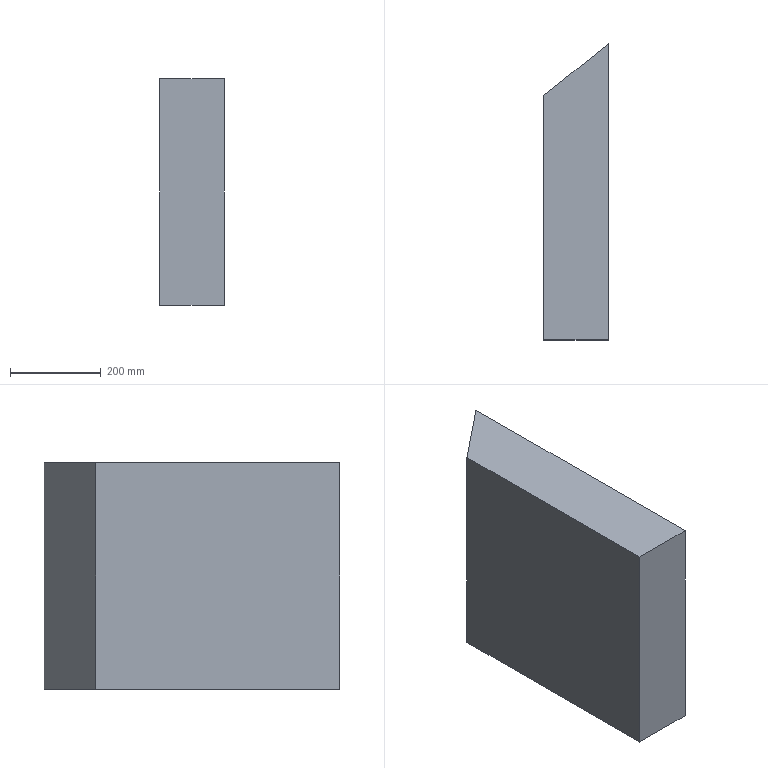Part | STEP file | S | 1 solid | 6 faces | box 142.095 x 652.75 x 500 mm | volume 42330846 mm3 | plane 6
STEP:
#1=CARTESIAN_POINT('',(0.,0.,0.));
#2=DIRECTION('',(0.,0.,1.));
#3=DIRECTION('',(1.,0.,0.));
#4=AXIS2_PLACEMENT_3D('',#1,#2,#3);
#5=CARTESIAN_POINT('',(0.,538.867,0.));
#6=VERTEX_POINT('',#5);
#7=CARTESIAN_POINT('',(0.,0.,0.));
#8=VERTEX_POINT('',#7);
#9=CARTESIAN_POINT('',(0.,286.117,0.));
#10=DIRECTION('',(0.,-1.,0.));
#11=VECTOR('',#10,1.);
#12=LINE('',#9,#11);
#13=CARTESIAN_POINT('',(0.,286.117,0.));
#14=DIRECTION('',(-1.,0.,0.));
#15=DIRECTION('',(0.,-1.,0.));
#16=AXIS2_PLACEMENT_3D('',#13,#14,#15);
#17=PLANE('',#16);
#18=CARTESIAN_POINT('',(0.,0.));
#19=DIRECTION('',(1.,0.));
#20=VECTOR('',#19,1.);
#21=LINE('',#18,#20);
#22=(GEOMETRIC_REPRESENTATION_CONTEXT(2)PARAMETRIC_REPRESENTATION_CONTEXT()REPRESENTATION_CONTEXT('',''));
#23=DEFINITIONAL_REPRESENTATION('',(#21),#22);
#24=PCURVE('',#17,#23);
#25=CARTESIAN_POINT('',(79.056,181.53,0.));
#26=DIRECTION('',(0.,0.,1.));
#27=DIRECTION('',(1.,0.,0.));
#28=AXIS2_PLACEMENT_3D('',#25,#26,#27);
#29=PLANE('',#28);
#30=CARTESIAN_POINT('',(-79.056,104.587));
#31=DIRECTION('',(0.,-1.));
#32=VECTOR('',#31,1.);
#33=LINE('',#30,#32);
#34=(GEOMETRIC_REPRESENTATION_CONTEXT(2)PARAMETRIC_REPRESENTATION_CONTEXT()REPRESENTATION_CONTEXT('',''));
#35=DEFINITIONAL_REPRESENTATION('',(#33),#34);
#36=PCURVE('',#29,#35);
#37=SURFACE_CURVE('',#12,(#24,#36),.PCURVE_S1.);
#38=EDGE_CURVE('',#6,#8,#37,.T.);
#39=ORIENTED_EDGE('',*,*,#38,.T.);
#40=CARTESIAN_POINT('',(0.,0.,500.));
#41=VERTEX_POINT('',#40);
#42=CARTESIAN_POINT('',(0.,0.,0.));
#43=DIRECTION('',(0.,0.,1.));
#44=VECTOR('',#43,1.);
#45=LINE('',#42,#44);
#46=CARTESIAN_POINT('',(286.117,0.));
#47=DIRECTION('',(0.,1.));
#48=VECTOR('',#47,1.);
#49=LINE('',#46,#48);
#50=(GEOMETRIC_REPRESENTATION_CONTEXT(2)PARAMETRIC_REPRESENTATION_CONTEXT()REPRESENTATION_CONTEXT('',''));
#51=DEFINITIONAL_REPRESENTATION('',(#49),#50);
#52=PCURVE('',#17,#51);
#53=CARTESIAN_POINT('',(0.,0.,0.));
#54=DIRECTION('',(0.,-1.,0.));
#55=DIRECTION('',(1.,0.,0.));
#56=AXIS2_PLACEMENT_3D('',#53,#54,#55);
#57=PLANE('',#56);
#58=CARTESIAN_POINT('',(0.,0.));
#59=DIRECTION('',(0.,1.));
#60=VECTOR('',#59,1.);
#61=LINE('',#58,#60);
#62=(GEOMETRIC_REPRESENTATION_CONTEXT(2)PARAMETRIC_REPRESENTATION_CONTEXT()REPRESENTATION_CONTEXT('',''));
#63=DEFINITIONAL_REPRESENTATION('',(#61),#62);
#64=PCURVE('',#57,#63);
#65=SURFACE_CURVE('',#45,(#52,#64),.PCURVE_S1.);
#66=EDGE_CURVE('',#8,#41,#65,.T.);
#67=ORIENTED_EDGE('',*,*,#66,.T.);
#68=CARTESIAN_POINT('',(0.,538.867,500.));
#69=VERTEX_POINT('',#68);
#70=CARTESIAN_POINT('',(0.,286.117,500.));
#71=DIRECTION('',(0.,-1.,0.));
#72=VECTOR('',#71,1.);
#73=LINE('',#70,#72);
#74=CARTESIAN_POINT('',(0.,500.));
#75=DIRECTION('',(1.,0.));
#76=VECTOR('',#75,1.);
#77=LINE('',#74,#76);
#78=(GEOMETRIC_REPRESENTATION_CONTEXT(2)PARAMETRIC_REPRESENTATION_CONTEXT()REPRESENTATION_CONTEXT('',''));
#79=DEFINITIONAL_REPRESENTATION('',(#77),#78);
#80=PCURVE('',#17,#79);
#81=CARTESIAN_POINT('',(79.056,181.53,500.));
#82=DIRECTION('',(0.,0.,1.));
#83=DIRECTION('',(1.,0.,0.));
#84=AXIS2_PLACEMENT_3D('',#81,#82,#83);
#85=PLANE('',#84);
#86=CARTESIAN_POINT('',(-79.056,104.587));
#87=DIRECTION('',(0.,-1.));
#88=VECTOR('',#87,1.);
#89=LINE('',#86,#88);
#90=(GEOMETRIC_REPRESENTATION_CONTEXT(2)PARAMETRIC_REPRESENTATION_CONTEXT()REPRESENTATION_CONTEXT('',''));
#91=DEFINITIONAL_REPRESENTATION('',(#89),#90);
#92=PCURVE('',#85,#91);
#93=SURFACE_CURVE('',#73,(#80,#92),.PCURVE_S1.);
#94=EDGE_CURVE('',#69,#41,#93,.T.);
#95=ORIENTED_EDGE('',*,*,#94,.F.);
#96=CARTESIAN_POINT('',(0.,538.867,0.));
#97=DIRECTION('',(0.,0.,1.));
#98=VECTOR('',#97,1.);
#99=LINE('',#96,#98);
#100=CARTESIAN_POINT('',(-252.75,0.));
#101=DIRECTION('',(0.,1.));
#102=VECTOR('',#101,1.);
#103=LINE('',#100,#102);
#104=(GEOMETRIC_REPRESENTATION_CONTEXT(2)PARAMETRIC_REPRESENTATION_CONTEXT()REPRESENTATION_CONTEXT('',''));
#105=DEFINITIONAL_REPRESENTATION('',(#103),#104);
#106=PCURVE('',#17,#105);
#107=CARTESIAN_POINT('',(142.095,652.75,0.));
#108=DIRECTION('',(-0.6254,0.7803,0.));
#109=DIRECTION('',(-0.7803,-0.6254,0.));
#110=AXIS2_PLACEMENT_3D('',#107,#108,#109);
#111=PLANE('',#110);
#112=CARTESIAN_POINT('',(182.1,0.));
#113=DIRECTION('',(0.,1.));
#114=VECTOR('',#113,1.);
#115=LINE('',#112,#114);
#116=(GEOMETRIC_REPRESENTATION_CONTEXT(2)PARAMETRIC_REPRESENTATION_CONTEXT()REPRESENTATION_CONTEXT('',''));
#117=DEFINITIONAL_REPRESENTATION('',(#115),#116);
#118=PCURVE('',#111,#117);
#119=SURFACE_CURVE('',#99,(#106,#118),.PCURVE_S1.);
#120=EDGE_CURVE('',#6,#69,#119,.T.);
#121=ORIENTED_EDGE('',*,*,#120,.F.);
#122=EDGE_LOOP('',(#39,#67,#95,#121));
#123=FACE_BOUND('',#122,.T.);
#124=ADVANCED_FACE('',(#123),#17,.T.);
#125=CARTESIAN_POINT('',(142.095,652.75,0.));
#126=VERTEX_POINT('',#125);
#127=CARTESIAN_POINT('',(142.095,652.75,0.));
#128=DIRECTION('',(-0.7803,-0.6254,0.));
#129=VECTOR('',#128,1.);
#130=LINE('',#127,#129);
#131=CARTESIAN_POINT('',(0.,0.));
#132=DIRECTION('',(1.,0.));
#133=VECTOR('',#132,1.);
#134=LINE('',#131,#133);
#135=(GEOMETRIC_REPRESENTATION_CONTEXT(2)PARAMETRIC_REPRESENTATION_CONTEXT()REPRESENTATION_CONTEXT('',''));
#136=DEFINITIONAL_REPRESENTATION('',(#134),#135);
#137=PCURVE('',#111,#136);
#138=CARTESIAN_POINT('',(63.039,471.22));
#139=DIRECTION('',(-0.7803,-0.6254));
#140=VECTOR('',#139,1.);
#141=LINE('',#138,#140);
#142=(GEOMETRIC_REPRESENTATION_CONTEXT(2)PARAMETRIC_REPRESENTATION_CONTEXT()REPRESENTATION_CONTEXT('',''));
#143=DEFINITIONAL_REPRESENTATION('',(#141),#142);
#144=PCURVE('',#29,#143);
#145=SURFACE_CURVE('',#130,(#137,#144),.PCURVE_S1.);
#146=EDGE_CURVE('',#126,#6,#145,.T.);
#147=ORIENTED_EDGE('',*,*,#146,.T.);
#148=ORIENTED_EDGE('',*,*,#120,.T.);
#149=CARTESIAN_POINT('',(142.095,652.75,500.));
#150=VERTEX_POINT('',#149);
#151=CARTESIAN_POINT('',(142.095,652.75,500.));
#152=DIRECTION('',(-0.7803,-0.6254,0.));
#153=VECTOR('',#152,1.);
#154=LINE('',#151,#153);
#155=CARTESIAN_POINT('',(0.,500.));
#156=DIRECTION('',(1.,0.));
#157=VECTOR('',#156,1.);
#158=LINE('',#155,#157);
#159=(GEOMETRIC_REPRESENTATION_CONTEXT(2)PARAMETRIC_REPRESENTATION_CONTEXT()REPRESENTATION_CONTEXT('',''));
#160=DEFINITIONAL_REPRESENTATION('',(#158),#159);
#161=PCURVE('',#111,#160);
#162=CARTESIAN_POINT('',(63.039,471.22));
#163=DIRECTION('',(-0.7803,-0.6254));
#164=VECTOR('',#163,1.);
#165=LINE('',#162,#164);
#166=(GEOMETRIC_REPRESENTATION_CONTEXT(2)PARAMETRIC_REPRESENTATION_CONTEXT()REPRESENTATION_CONTEXT('',''));
#167=DEFINITIONAL_REPRESENTATION('',(#165),#166);
#168=PCURVE('',#85,#167);
#169=SURFACE_CURVE('',#154,(#161,#168),.PCURVE_S1.);
#170=EDGE_CURVE('',#150,#69,#169,.T.);
#171=ORIENTED_EDGE('',*,*,#170,.F.);
#172=CARTESIAN_POINT('',(142.095,652.75,0.));
#173=DIRECTION('',(0.,0.,1.));
#174=VECTOR('',#173,1.);
#175=LINE('',#172,#174);
#176=CARTESIAN_POINT('',(0.,0.));
#177=DIRECTION('',(0.,1.));
#178=VECTOR('',#177,1.);
#179=LINE('',#176,#178);
#180=(GEOMETRIC_REPRESENTATION_CONTEXT(2)PARAMETRIC_REPRESENTATION_CONTEXT()REPRESENTATION_CONTEXT('',''));
#181=DEFINITIONAL_REPRESENTATION('',(#179),#180);
#182=PCURVE('',#111,#181);
#183=CARTESIAN_POINT('',(142.095,0.,0.));
#184=DIRECTION('',(1.,0.,0.));
#185=DIRECTION('',(0.,1.,0.));
#186=AXIS2_PLACEMENT_3D('',#183,#184,#185);
#187=PLANE('',#186);
#188=CARTESIAN_POINT('',(652.75,0.));
#189=DIRECTION('',(0.,1.));
#190=VECTOR('',#189,1.);
#191=LINE('',#188,#190);
#192=(GEOMETRIC_REPRESENTATION_CONTEXT(2)PARAMETRIC_REPRESENTATION_CONTEXT()REPRESENTATION_CONTEXT('',''));
#193=DEFINITIONAL_REPRESENTATION('',(#191),#192);
#194=PCURVE('',#187,#193);
#195=SURFACE_CURVE('',#175,(#182,#194),.PCURVE_S1.);
#196=EDGE_CURVE('',#126,#150,#195,.T.);
#197=ORIENTED_EDGE('',*,*,#196,.F.);
#198=EDGE_LOOP('',(#147,#148,#171,#197));
#199=FACE_BOUND('',#198,.T.);
#200=ADVANCED_FACE('',(#199),#111,.T.);
#201=CARTESIAN_POINT('',(142.095,0.,0.));
#202=VERTEX_POINT('',#201);
#203=CARTESIAN_POINT('',(142.095,0.,0.));
#204=DIRECTION('',(0.,1.,0.));
#205=VECTOR('',#204,1.);
#206=LINE('',#203,#205);
#207=CARTESIAN_POINT('',(0.,0.));
#208=DIRECTION('',(1.,0.));
#209=VECTOR('',#208,1.);
#210=LINE('',#207,#209);
#211=(GEOMETRIC_REPRESENTATION_CONTEXT(2)PARAMETRIC_REPRESENTATION_CONTEXT()REPRESENTATION_CONTEXT('',''));
#212=DEFINITIONAL_REPRESENTATION('',(#210),#211);
#213=PCURVE('',#187,#212);
#214=CARTESIAN_POINT('',(63.039,-181.53));
#215=DIRECTION('',(0.,1.));
#216=VECTOR('',#215,1.);
#217=LINE('',#214,#216);
#218=(GEOMETRIC_REPRESENTATION_CONTEXT(2)PARAMETRIC_REPRESENTATION_CONTEXT()REPRESENTATION_CONTEXT('',''));
#219=DEFINITIONAL_REPRESENTATION('',(#217),#218);
#220=PCURVE('',#29,#219);
#221=SURFACE_CURVE('',#206,(#213,#220),.PCURVE_S1.);
#222=EDGE_CURVE('',#202,#126,#221,.T.);
#223=ORIENTED_EDGE('',*,*,#222,.T.);
#224=ORIENTED_EDGE('',*,*,#196,.T.);
#225=CARTESIAN_POINT('',(142.095,0.,500.));
#226=VERTEX_POINT('',#225);
#227=CARTESIAN_POINT('',(142.095,0.,500.));
#228=DIRECTION('',(0.,1.,0.));
#229=VECTOR('',#228,1.);
#230=LINE('',#227,#229);
#231=CARTESIAN_POINT('',(0.,500.));
#232=DIRECTION('',(1.,0.));
#233=VECTOR('',#232,1.);
#234=LINE('',#231,#233);
#235=(GEOMETRIC_REPRESENTATION_CONTEXT(2)PARAMETRIC_REPRESENTATION_CONTEXT()REPRESENTATION_CONTEXT('',''));
#236=DEFINITIONAL_REPRESENTATION('',(#234),#235);
#237=PCURVE('',#187,#236);
#238=CARTESIAN_POINT('',(63.039,-181.53));
#239=DIRECTION('',(0.,1.));
#240=VECTOR('',#239,1.);
#241=LINE('',#238,#240);
#242=(GEOMETRIC_REPRESENTATION_CONTEXT(2)PARAMETRIC_REPRESENTATION_CONTEXT()REPRESENTATION_CONTEXT('',''));
#243=DEFINITIONAL_REPRESENTATION('',(#241),#242);
#244=PCURVE('',#85,#243);
#245=SURFACE_CURVE('',#230,(#237,#244),.PCURVE_S1.);
#246=EDGE_CURVE('',#226,#150,#245,.T.);
#247=ORIENTED_EDGE('',*,*,#246,.F.);
#248=CARTESIAN_POINT('',(142.095,0.,0.));
#249=DIRECTION('',(0.,0.,1.));
#250=VECTOR('',#249,1.);
#251=LINE('',#248,#250);
#252=CARTESIAN_POINT('',(0.,0.));
#253=DIRECTION('',(0.,1.));
#254=VECTOR('',#253,1.);
#255=LINE('',#252,#254);
#256=(GEOMETRIC_REPRESENTATION_CONTEXT(2)PARAMETRIC_REPRESENTATION_CONTEXT()REPRESENTATION_CONTEXT('',''));
#257=DEFINITIONAL_REPRESENTATION('',(#255),#256);
#258=PCURVE('',#187,#257);
#259=CARTESIAN_POINT('',(142.095,0.));
#260=DIRECTION('',(0.,1.));
#261=VECTOR('',#260,1.);
#262=LINE('',#259,#261);
#263=(GEOMETRIC_REPRESENTATION_CONTEXT(2)PARAMETRIC_REPRESENTATION_CONTEXT()REPRESENTATION_CONTEXT('',''));
#264=DEFINITIONAL_REPRESENTATION('',(#262),#263);
#265=PCURVE('',#57,#264);
#266=SURFACE_CURVE('',#251,(#258,#265),.PCURVE_S1.);
#267=EDGE_CURVE('',#202,#226,#266,.T.);
#268=ORIENTED_EDGE('',*,*,#267,.F.);
#269=EDGE_LOOP('',(#223,#224,#247,#268));
#270=FACE_BOUND('',#269,.T.);
#271=ADVANCED_FACE('',(#270),#187,.T.);
#272=CARTESIAN_POINT('',(0.,0.,0.));
#273=DIRECTION('',(1.,0.,0.));
#274=VECTOR('',#273,1.);
#275=LINE('',#272,#274);
#276=CARTESIAN_POINT('',(0.,0.));
#277=DIRECTION('',(1.,0.));
#278=VECTOR('',#277,1.);
#279=LINE('',#276,#278);
#280=(GEOMETRIC_REPRESENTATION_CONTEXT(2)PARAMETRIC_REPRESENTATION_CONTEXT()REPRESENTATION_CONTEXT('',''));
#281=DEFINITIONAL_REPRESENTATION('',(#279),#280);
#282=PCURVE('',#57,#281);
#283=CARTESIAN_POINT('',(-79.056,-181.53));
#284=DIRECTION('',(1.,0.));
#285=VECTOR('',#284,1.);
#286=LINE('',#283,#285);
#287=(GEOMETRIC_REPRESENTATION_CONTEXT(2)PARAMETRIC_REPRESENTATION_CONTEXT()REPRESENTATION_CONTEXT('',''));
#288=DEFINITIONAL_REPRESENTATION('',(#286),#287);
#289=PCURVE('',#29,#288);
#290=SURFACE_CURVE('',#275,(#282,#289),.PCURVE_S1.);
#291=EDGE_CURVE('',#8,#202,#290,.T.);
#292=ORIENTED_EDGE('',*,*,#291,.T.);
#293=ORIENTED_EDGE('',*,*,#267,.T.);
#294=CARTESIAN_POINT('',(0.,0.,500.));
#295=DIRECTION('',(1.,0.,0.));
#296=VECTOR('',#295,1.);
#297=LINE('',#294,#296);
#298=CARTESIAN_POINT('',(0.,500.));
#299=DIRECTION('',(1.,0.));
#300=VECTOR('',#299,1.);
#301=LINE('',#298,#300);
#302=(GEOMETRIC_REPRESENTATION_CONTEXT(2)PARAMETRIC_REPRESENTATION_CONTEXT()REPRESENTATION_CONTEXT('',''));
#303=DEFINITIONAL_REPRESENTATION('',(#301),#302);
#304=PCURVE('',#57,#303);
#305=CARTESIAN_POINT('',(-79.056,-181.53));
#306=DIRECTION('',(1.,0.));
#307=VECTOR('',#306,1.);
#308=LINE('',#305,#307);
#309=(GEOMETRIC_REPRESENTATION_CONTEXT(2)PARAMETRIC_REPRESENTATION_CONTEXT()REPRESENTATION_CONTEXT('',''));
#310=DEFINITIONAL_REPRESENTATION('',(#308),#309);
#311=PCURVE('',#85,#310);
#312=SURFACE_CURVE('',#297,(#304,#311),.PCURVE_S1.);
#313=EDGE_CURVE('',#41,#226,#312,.T.);
#314=ORIENTED_EDGE('',*,*,#313,.F.);
#315=ORIENTED_EDGE('',*,*,#66,.F.);
#316=EDGE_LOOP('',(#292,#293,#314,#315));
#317=FACE_BOUND('',#316,.T.);
#318=ADVANCED_FACE('',(#317),#57,.T.);
#319=ORIENTED_EDGE('',*,*,#313,.T.);
#320=ORIENTED_EDGE('',*,*,#246,.T.);
#321=ORIENTED_EDGE('',*,*,#170,.T.);
#322=ORIENTED_EDGE('',*,*,#94,.T.);
#323=EDGE_LOOP('',(#319,#320,#321,#322));
#324=FACE_BOUND('',#323,.T.);
#325=ADVANCED_FACE('',(#324),#85,.T.);
#326=ORIENTED_EDGE('',*,*,#291,.F.);
#327=ORIENTED_EDGE('',*,*,#38,.F.);
#328=ORIENTED_EDGE('',*,*,#146,.F.);
#329=ORIENTED_EDGE('',*,*,#222,.F.);
#330=EDGE_LOOP('',(#326,#327,#328,#329));
#331=FACE_BOUND('',#330,.T.);
#332=ADVANCED_FACE('',(#331),#29,.F.);
#333=CLOSED_SHELL('',(#124,#200,#271,#318,#325,#332));
#334=MANIFOLD_SOLID_BREP('',#333);
#335=(LENGTH_UNIT()NAMED_UNIT(*)SI_UNIT(.MILLI.,.METRE.));
#336=UNCERTAINTY_MEASURE_WITH_UNIT(LENGTH_MEASURE(0.0000001),#335,'','');
#337=(NAMED_UNIT(*)PLANE_ANGLE_UNIT()SI_UNIT($,.RADIAN.));
#338=(NAMED_UNIT(*)SI_UNIT($,.STERADIAN.)SOLID_ANGLE_UNIT());
#339=(GEOMETRIC_REPRESENTATION_CONTEXT(3)GLOBAL_UNCERTAINTY_ASSIGNED_CONTEXT((#336))GLOBAL_UNIT_ASSIGNED_CONTEXT((#335,#337,#338))REPRESENTATION_CONTEXT('',''));
#340=ADVANCED_BREP_SHAPE_REPRESENTATION('',(#4,#334),#339);